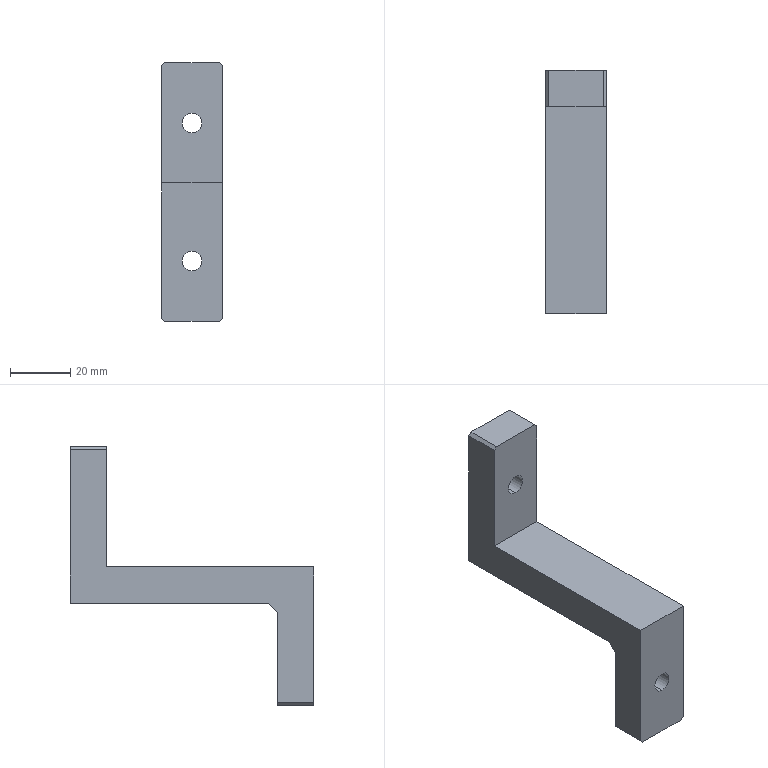Part | NX | features BREP 1 | 1 solid | 25 faces | box 20 x 81 x 86 mm | volume 35618 mm3 | plane 17 | cylinder 8 | commonest cylinder face diameters 6.6 x4 11 x4
STEP:
#1=CARTESIAN_POINT('',(9.,12.,0.));
#2=VERTEX_POINT('',#1);
#3=CARTESIAN_POINT('',(10.,12.,-1.));
#4=VERTEX_POINT('',#3);
#5=CARTESIAN_POINT('',(10.,12.,-1.));
#6=DIRECTION('',(0.7071,0.,-0.7071));
#7=VECTOR('',#6,1000.);
#8=LINE('',#5,#7);
#9=EDGE_CURVE('',#2,#4,#8,.T.);
#10=ORIENTED_EDGE('',*,*,#9,.F.);
#11=CARTESIAN_POINT('',(9.,0.,0.));
#12=VERTEX_POINT('',#11);
#13=CARTESIAN_POINT('',(9.,12.,0.));
#14=DIRECTION('',(0.,1.,0.));
#15=VECTOR('',#14,1000.);
#16=LINE('',#13,#15);
#17=EDGE_CURVE('',#12,#2,#16,.T.);
#18=ORIENTED_EDGE('',*,*,#17,.F.);
#19=CARTESIAN_POINT('',(10.,0.,-1.));
#20=VERTEX_POINT('',#19);
#21=CARTESIAN_POINT('',(10.,0.,-1.));
#22=DIRECTION('',(-0.7071,0.,0.7071));
#23=VECTOR('',#22,1000.);
#24=LINE('',#21,#23);
#25=EDGE_CURVE('',#20,#12,#24,.T.);
#26=ORIENTED_EDGE('',*,*,#25,.F.);
#27=CARTESIAN_POINT('',(10.,0.,-1.));
#28=DIRECTION('',(0.,-1.,0.));
#29=VECTOR('',#28,1000.);
#30=LINE('',#27,#29);
#31=EDGE_CURVE('',#4,#20,#30,.T.);
#32=ORIENTED_EDGE('',*,*,#31,.F.);
#33=EDGE_LOOP('',(#10,#18,#26,#32));
#34=FACE_BOUND('',#33,.T.);
#35=CARTESIAN_POINT('',(10.,0.,-1.));
#36=DIRECTION('',(0.7071,0.,0.7071));
#37=DIRECTION('',(0.,1.,0.));
#38=AXIS2_PLACEMENT_3D('',#35,#36,#37);
#39=PLANE('',#38);
#40=ADVANCED_FACE('',(#34),#39,.T.);
#41=CARTESIAN_POINT('',(-10.,12.,-1.));
#42=VERTEX_POINT('',#41);
#43=CARTESIAN_POINT('',(-9.,12.,0.));
#44=VERTEX_POINT('',#43);
#45=CARTESIAN_POINT('',(-9.,12.,0.));
#46=DIRECTION('',(0.7071,0.,0.7071));
#47=VECTOR('',#46,1000.);
#48=LINE('',#45,#47);
#49=EDGE_CURVE('',#42,#44,#48,.T.);
#50=ORIENTED_EDGE('',*,*,#49,.F.);
#51=CARTESIAN_POINT('',(-10.,0.,-1.));
#52=VERTEX_POINT('',#51);
#53=CARTESIAN_POINT('',(-10.,0.,-1.));
#54=DIRECTION('',(0.,1.,0.));
#55=VECTOR('',#54,1000.);
#56=LINE('',#53,#55);
#57=EDGE_CURVE('',#52,#42,#56,.T.);
#58=ORIENTED_EDGE('',*,*,#57,.F.);
#59=CARTESIAN_POINT('',(-9.,0.,0.));
#60=VERTEX_POINT('',#59);
#61=CARTESIAN_POINT('',(-9.,0.,0.));
#62=DIRECTION('',(-0.7071,0.,-0.7071));
#63=VECTOR('',#62,1000.);
#64=LINE('',#61,#63);
#65=EDGE_CURVE('',#60,#52,#64,.T.);
#66=ORIENTED_EDGE('',*,*,#65,.F.);
#67=CARTESIAN_POINT('',(-9.,12.,0.));
#68=DIRECTION('',(0.,-1.,0.));
#69=VECTOR('',#68,1000.);
#70=LINE('',#67,#69);
#71=EDGE_CURVE('',#44,#60,#70,.T.);
#72=ORIENTED_EDGE('',*,*,#71,.F.);
#73=EDGE_LOOP('',(#50,#58,#66,#72));
#74=FACE_BOUND('',#73,.T.);
#75=CARTESIAN_POINT('',(-9.,12.,0.));
#76=DIRECTION('',(0.7071,0.,-0.7071));
#77=DIRECTION('',(0.,-1.,0.));
#78=AXIS2_PLACEMENT_3D('',#75,#76,#77);
#79=PLANE('',#78);
#80=ADVANCED_FACE('',(#74),#79,.F.);
#81=CARTESIAN_POINT('',(9.,-69.,-86.));
#82=VERTEX_POINT('',#81);
#83=CARTESIAN_POINT('',(10.,-69.,-85.));
#84=VERTEX_POINT('',#83);
#85=CARTESIAN_POINT('',(10.,-69.,-85.));
#86=DIRECTION('',(0.7071,0.,0.7071));
#87=VECTOR('',#86,1000.);
#88=LINE('',#85,#87);
#89=EDGE_CURVE('',#82,#84,#88,.T.);
#90=ORIENTED_EDGE('',*,*,#89,.F.);
#91=CARTESIAN_POINT('',(9.,-57.,-86.));
#92=VERTEX_POINT('',#91);
#93=CARTESIAN_POINT('',(9.,-69.,-86.));
#94=DIRECTION('',(0.,-1.,0.));
#95=VECTOR('',#94,1000.);
#96=LINE('',#93,#95);
#97=EDGE_CURVE('',#92,#82,#96,.T.);
#98=ORIENTED_EDGE('',*,*,#97,.F.);
#99=CARTESIAN_POINT('',(10.,-57.,-85.));
#100=VERTEX_POINT('',#99);
#101=CARTESIAN_POINT('',(10.,-57.,-85.));
#102=DIRECTION('',(-0.7071,0.,-0.7071));
#103=VECTOR('',#102,1000.);
#104=LINE('',#101,#103);
#105=EDGE_CURVE('',#100,#92,#104,.T.);
#106=ORIENTED_EDGE('',*,*,#105,.F.);
#107=CARTESIAN_POINT('',(10.,-57.,-85.));
#108=DIRECTION('',(0.,1.,0.));
#109=VECTOR('',#108,1000.);
#110=LINE('',#107,#109);
#111=EDGE_CURVE('',#84,#100,#110,.T.);
#112=ORIENTED_EDGE('',*,*,#111,.F.);
#113=EDGE_LOOP('',(#90,#98,#106,#112));
#114=FACE_BOUND('',#113,.T.);
#115=CARTESIAN_POINT('',(10.,0.,-85.));
#116=DIRECTION('',(0.7071,0.,-0.7071));
#117=DIRECTION('',(0.,-1.,0.));
#118=AXIS2_PLACEMENT_3D('',#115,#116,#117);
#119=PLANE('',#118);
#120=ADVANCED_FACE('',(#114),#119,.T.);
#121=CARTESIAN_POINT('',(-10.,-69.,-85.));
#122=VERTEX_POINT('',#121);
#123=CARTESIAN_POINT('',(-9.,-69.,-86.));
#124=VERTEX_POINT('',#123);
#125=CARTESIAN_POINT('',(-9.,-69.,-86.));
#126=DIRECTION('',(0.7071,0.,-0.7071));
#127=VECTOR('',#126,1000.);
#128=LINE('',#125,#127);
#129=EDGE_CURVE('',#122,#124,#128,.T.);
#130=ORIENTED_EDGE('',*,*,#129,.F.);
#131=CARTESIAN_POINT('',(-10.,-57.,-85.));
#132=VERTEX_POINT('',#131);
#133=CARTESIAN_POINT('',(-10.,0.,-85.));
#134=DIRECTION('',(0.,-1.,0.));
#135=VECTOR('',#134,1000.);
#136=LINE('',#133,#135);
#137=EDGE_CURVE('',#132,#122,#136,.T.);
#138=ORIENTED_EDGE('',*,*,#137,.F.);
#139=CARTESIAN_POINT('',(-9.,-57.,-86.));
#140=VERTEX_POINT('',#139);
#141=CARTESIAN_POINT('',(-9.,-57.,-86.));
#142=DIRECTION('',(-0.7071,0.,0.7071));
#143=VECTOR('',#142,1000.);
#144=LINE('',#141,#143);
#145=EDGE_CURVE('',#140,#132,#144,.T.);
#146=ORIENTED_EDGE('',*,*,#145,.F.);
#147=CARTESIAN_POINT('',(-9.,-69.,-86.));
#148=DIRECTION('',(0.,1.,0.));
#149=VECTOR('',#148,1000.);
#150=LINE('',#147,#149);
#151=EDGE_CURVE('',#124,#140,#150,.T.);
#152=ORIENTED_EDGE('',*,*,#151,.F.);
#153=EDGE_LOOP('',(#130,#138,#146,#152));
#154=FACE_BOUND('',#153,.T.);
#155=CARTESIAN_POINT('',(-9.,-69.,-86.));
#156=DIRECTION('',(0.7071,0.,0.7071));
#157=DIRECTION('',(0.,1.,0.));
#158=AXIS2_PLACEMENT_3D('',#155,#156,#157);
#159=PLANE('',#158);
#160=ADVANCED_FACE('',(#154),#159,.F.);
#161=CARTESIAN_POINT('',(0.,-57.,-71.5));
#162=VERTEX_POINT('',#161);
#163=CARTESIAN_POINT('',(0.,-63.8,-71.5));
#164=VERTEX_POINT('',#163);
#165=CARTESIAN_POINT('',(0.,-57.,-71.5));
#166=DIRECTION('',(0.,1.,0.));
#167=VECTOR('',#166,1000.);
#168=LINE('',#165,#167);
#169=EDGE_CURVE('',#162,#164,#168,.F.);
#170=ORIENTED_EDGE('',*,*,#169,.T.);
#171=CARTESIAN_POINT('',(0.,-63.8,-60.5));
#172=VERTEX_POINT('',#171);
#173=CARTESIAN_POINT('',(0.,-63.8,-66.));
#174=DIRECTION('',(0.,1.,0.));
#175=DIRECTION('',(0.,0.,1.));
#176=AXIS2_PLACEMENT_3D('',#173,#174,#175);
#177=CIRCLE('',#176,5.5);
#178=EDGE_CURVE('',#172,#164,#177,.T.);
#179=ORIENTED_EDGE('',*,*,#178,.F.);
#180=CARTESIAN_POINT('',(0.,-57.,-60.5));
#181=VERTEX_POINT('',#180);
#182=CARTESIAN_POINT('',(0.,-57.,-60.5));
#183=DIRECTION('',(0.,1.,0.));
#184=VECTOR('',#183,1000.);
#185=LINE('',#182,#184);
#186=EDGE_CURVE('',#181,#172,#185,.F.);
#187=ORIENTED_EDGE('',*,*,#186,.F.);
#188=CARTESIAN_POINT('',(0.,-57.,-66.));
#189=DIRECTION('',(0.,1.,0.));
#190=DIRECTION('',(0.,0.,1.));
#191=AXIS2_PLACEMENT_3D('',#188,#189,#190);
#192=CIRCLE('',#191,5.5);
#193=EDGE_CURVE('',#181,#162,#192,.T.);
#194=ORIENTED_EDGE('',*,*,#193,.T.);
#195=EDGE_LOOP('',(#170,#179,#187,#194));
#196=FACE_BOUND('',#195,.T.);
#197=CARTESIAN_POINT('',(0.,-57.,-66.));
#198=DIRECTION('',(0.,1.,0.));
#199=DIRECTION('',(0.,0.,1.));
#200=AXIS2_PLACEMENT_3D('',#197,#198,#199);
#201=CYLINDRICAL_SURFACE('',#200,5.5);
#202=ADVANCED_FACE('',(#196),#201,.F.);
#203=ORIENTED_EDGE('',*,*,#178,.T.);
#204=CARTESIAN_POINT('',(0.,-63.8,-66.));
#205=DIRECTION('',(0.,1.,0.));
#206=DIRECTION('',(0.,0.,1.));
#207=AXIS2_PLACEMENT_3D('',#204,#205,#206);
#208=CIRCLE('',#207,5.5);
#209=EDGE_CURVE('',#164,#172,#208,.T.);
#210=ORIENTED_EDGE('',*,*,#209,.T.);
#211=EDGE_LOOP('',(#203,#210));
#212=FACE_BOUND('',#211,.T.);
#213=CARTESIAN_POINT('',(0.,-63.8,-62.7));
#214=VERTEX_POINT('',#213);
#215=CARTESIAN_POINT('',(0.,-63.8,-69.3));
#216=VERTEX_POINT('',#215);
#217=CARTESIAN_POINT('',(0.,-63.8,-66.));
#218=DIRECTION('',(0.,1.,0.));
#219=DIRECTION('',(0.,0.,1.));
#220=AXIS2_PLACEMENT_3D('',#217,#218,#219);
#221=CIRCLE('',#220,3.3);
#222=EDGE_CURVE('',#214,#216,#221,.T.);
#223=ORIENTED_EDGE('',*,*,#222,.F.);
#224=CARTESIAN_POINT('',(0.,-63.8,-66.));
#225=DIRECTION('',(0.,1.,0.));
#226=DIRECTION('',(0.,0.,1.));
#227=AXIS2_PLACEMENT_3D('',#224,#225,#226);
#228=CIRCLE('',#227,3.3);
#229=EDGE_CURVE('',#216,#214,#228,.T.);
#230=ORIENTED_EDGE('',*,*,#229,.F.);
#231=EDGE_LOOP('',(#223,#230));
#232=FACE_BOUND('',#231,.T.);
#233=CARTESIAN_POINT('',(3.3,-63.8,-66.));
#234=DIRECTION('',(0.,-1.,0.));
#235=DIRECTION('',(0.,0.,-1.));
#236=AXIS2_PLACEMENT_3D('',#233,#234,#235);
#237=PLANE('',#236);
#238=ADVANCED_FACE('',(#212,#232),#237,.F.);
#239=CARTESIAN_POINT('',(0.,-69.,-69.3));
#240=VERTEX_POINT('',#239);
#241=CARTESIAN_POINT('',(0.,-57.,-69.3));
#242=DIRECTION('',(0.,1.,0.));
#243=VECTOR('',#242,1000.);
#244=LINE('',#241,#243);
#245=EDGE_CURVE('',#216,#240,#244,.F.);
#246=ORIENTED_EDGE('',*,*,#245,.T.);
#247=CARTESIAN_POINT('',(0.,-69.,-62.7));
#248=VERTEX_POINT('',#247);
#249=CARTESIAN_POINT('',(0.,-69.,-66.));
#250=DIRECTION('',(0.,1.,0.));
#251=DIRECTION('',(0.,0.,1.));
#252=AXIS2_PLACEMENT_3D('',#249,#250,#251);
#253=CIRCLE('',#252,3.3);
#254=EDGE_CURVE('',#248,#240,#253,.T.);
#255=ORIENTED_EDGE('',*,*,#254,.F.);
#256=CARTESIAN_POINT('',(0.,-57.,-62.7));
#257=DIRECTION('',(0.,1.,0.));
#258=VECTOR('',#257,1000.);
#259=LINE('',#256,#258);
#260=EDGE_CURVE('',#214,#248,#259,.F.);
#261=ORIENTED_EDGE('',*,*,#260,.F.);
#262=ORIENTED_EDGE('',*,*,#222,.T.);
#263=EDGE_LOOP('',(#246,#255,#261,#262));
#264=FACE_BOUND('',#263,.T.);
#265=CARTESIAN_POINT('',(0.,-57.,-66.));
#266=DIRECTION('',(0.,1.,0.));
#267=DIRECTION('',(0.,0.,1.));
#268=AXIS2_PLACEMENT_3D('',#265,#266,#267);
#269=CYLINDRICAL_SURFACE('',#268,3.3);
#270=ADVANCED_FACE('',(#264),#269,.F.);
#271=CARTESIAN_POINT('',(10.,-57.,-55.));
#272=VERTEX_POINT('',#271);
#273=CARTESIAN_POINT('',(10.,-54.,-52.));
#274=VERTEX_POINT('',#273);
#275=CARTESIAN_POINT('',(10.,-54.,-52.));
#276=DIRECTION('',(0.,0.7071,0.7071));
#277=VECTOR('',#276,1000.);
#278=LINE('',#275,#277);
#279=EDGE_CURVE('',#272,#274,#278,.T.);
#280=ORIENTED_EDGE('',*,*,#279,.F.);
#281=CARTESIAN_POINT('',(-10.,-57.,-55.));
#282=VERTEX_POINT('',#281);
#283=CARTESIAN_POINT('',(10.,-57.,-55.));
#284=DIRECTION('',(1.,0.,0.));
#285=VECTOR('',#284,1000.);
#286=LINE('',#283,#285);
#287=EDGE_CURVE('',#282,#272,#286,.T.);
#288=ORIENTED_EDGE('',*,*,#287,.F.);
#289=CARTESIAN_POINT('',(-10.,-54.,-52.));
#290=VERTEX_POINT('',#289);
#291=CARTESIAN_POINT('',(-10.,-1.,1.));
#292=DIRECTION('',(0.,-0.7071,-0.7071));
#293=VECTOR('',#292,1000.);
#294=LINE('',#291,#293);
#295=EDGE_CURVE('',#290,#282,#294,.T.);
#296=ORIENTED_EDGE('',*,*,#295,.F.);
#297=CARTESIAN_POINT('',(-10.,-54.,-52.));
#298=DIRECTION('',(-1.,0.,0.));
#299=VECTOR('',#298,1000.);
#300=LINE('',#297,#299);
#301=EDGE_CURVE('',#274,#290,#300,.T.);
#302=ORIENTED_EDGE('',*,*,#301,.F.);
#303=EDGE_LOOP('',(#280,#288,#296,#302));
#304=FACE_BOUND('',#303,.T.);
#305=CARTESIAN_POINT('',(10.,-54.,-52.));
#306=DIRECTION('',(0.,0.7071,-0.7071));
#307=DIRECTION('',(1.,0.,0.));
#308=AXIS2_PLACEMENT_3D('',#305,#306,#307);
#309=PLANE('',#308);
#310=ADVANCED_FACE('',(#304),#309,.T.);
#311=CARTESIAN_POINT('',(0.,12.,-25.5));
#312=VERTEX_POINT('',#311);
#313=CARTESIAN_POINT('',(0.,5.2,-25.5));
#314=VERTEX_POINT('',#313);
#315=CARTESIAN_POINT('',(0.,12.,-25.5));
#316=DIRECTION('',(0.,1.,0.));
#317=VECTOR('',#316,1000.);
#318=LINE('',#315,#317);
#319=EDGE_CURVE('',#312,#314,#318,.F.);
#320=ORIENTED_EDGE('',*,*,#319,.T.);
#321=CARTESIAN_POINT('',(0.,5.2,-14.5));
#322=VERTEX_POINT('',#321);
#323=CARTESIAN_POINT('',(0.,5.2,-20.));
#324=DIRECTION('',(0.,1.,0.));
#325=DIRECTION('',(0.,0.,1.));
#326=AXIS2_PLACEMENT_3D('',#323,#324,#325);
#327=CIRCLE('',#326,5.5);
#328=EDGE_CURVE('',#322,#314,#327,.T.);
#329=ORIENTED_EDGE('',*,*,#328,.F.);
#330=CARTESIAN_POINT('',(0.,12.,-14.5));
#331=VERTEX_POINT('',#330);
#332=CARTESIAN_POINT('',(0.,12.,-14.5));
#333=DIRECTION('',(0.,1.,0.));
#334=VECTOR('',#333,1000.);
#335=LINE('',#332,#334);
#336=EDGE_CURVE('',#331,#322,#335,.F.);
#337=ORIENTED_EDGE('',*,*,#336,.F.);
#338=CARTESIAN_POINT('',(0.,12.,-20.));
#339=DIRECTION('',(0.,1.,0.));
#340=DIRECTION('',(0.,0.,1.));
#341=AXIS2_PLACEMENT_3D('',#338,#339,#340);
#342=CIRCLE('',#341,5.5);
#343=EDGE_CURVE('',#331,#312,#342,.T.);
#344=ORIENTED_EDGE('',*,*,#343,.T.);
#345=EDGE_LOOP('',(#320,#329,#337,#344));
#346=FACE_BOUND('',#345,.T.);
#347=CARTESIAN_POINT('',(0.,12.,-20.));
#348=DIRECTION('',(0.,1.,0.));
#349=DIRECTION('',(0.,0.,1.));
#350=AXIS2_PLACEMENT_3D('',#347,#348,#349);
#351=CYLINDRICAL_SURFACE('',#350,5.5);
#352=ADVANCED_FACE('',(#346),#351,.F.);
#353=ORIENTED_EDGE('',*,*,#328,.T.);
#354=CARTESIAN_POINT('',(0.,5.2,-20.));
#355=DIRECTION('',(0.,1.,0.));
#356=DIRECTION('',(0.,0.,1.));
#357=AXIS2_PLACEMENT_3D('',#354,#355,#356);
#358=CIRCLE('',#357,5.5);
#359=EDGE_CURVE('',#314,#322,#358,.T.);
#360=ORIENTED_EDGE('',*,*,#359,.T.);
#361=EDGE_LOOP('',(#353,#360));
#362=FACE_BOUND('',#361,.T.);
#363=CARTESIAN_POINT('',(0.,5.2,-16.7));
#364=VERTEX_POINT('',#363);
#365=CARTESIAN_POINT('',(0.,5.2,-23.3));
#366=VERTEX_POINT('',#365);
#367=CARTESIAN_POINT('',(0.,5.2,-20.));
#368=DIRECTION('',(0.,1.,0.));
#369=DIRECTION('',(0.,0.,1.));
#370=AXIS2_PLACEMENT_3D('',#367,#368,#369);
#371=CIRCLE('',#370,3.3);
#372=EDGE_CURVE('',#364,#366,#371,.T.);
#373=ORIENTED_EDGE('',*,*,#372,.F.);
#374=CARTESIAN_POINT('',(0.,5.2,-20.));
#375=DIRECTION('',(0.,1.,0.));
#376=DIRECTION('',(0.,0.,1.));
#377=AXIS2_PLACEMENT_3D('',#374,#375,#376);
#378=CIRCLE('',#377,3.3);
#379=EDGE_CURVE('',#366,#364,#378,.T.);
#380=ORIENTED_EDGE('',*,*,#379,.F.);
#381=EDGE_LOOP('',(#373,#380));
#382=FACE_BOUND('',#381,.T.);
#383=CARTESIAN_POINT('',(3.3,5.2,-20.));
#384=DIRECTION('',(0.,-1.,0.));
#385=DIRECTION('',(0.,0.,-1.));
#386=AXIS2_PLACEMENT_3D('',#383,#384,#385);
#387=PLANE('',#386);
#388=ADVANCED_FACE('',(#362,#382),#387,.F.);
#389=CARTESIAN_POINT('',(0.,0.,-23.3));
#390=VERTEX_POINT('',#389);
#391=CARTESIAN_POINT('',(0.,12.,-23.3));
#392=DIRECTION('',(0.,1.,0.));
#393=VECTOR('',#392,1000.);
#394=LINE('',#391,#393);
#395=EDGE_CURVE('',#366,#390,#394,.F.);
#396=ORIENTED_EDGE('',*,*,#395,.T.);
#397=CARTESIAN_POINT('',(0.,0.,-16.7));
#398=VERTEX_POINT('',#397);
#399=CARTESIAN_POINT('',(0.,0.,-20.));
#400=DIRECTION('',(0.,1.,0.));
#401=DIRECTION('',(0.,0.,1.));
#402=AXIS2_PLACEMENT_3D('',#399,#400,#401);
#403=CIRCLE('',#402,3.3);
#404=EDGE_CURVE('',#398,#390,#403,.T.);
#405=ORIENTED_EDGE('',*,*,#404,.F.);
#406=CARTESIAN_POINT('',(0.,12.,-16.7));
#407=DIRECTION('',(0.,1.,0.));
#408=VECTOR('',#407,1000.);
#409=LINE('',#406,#408);
#410=EDGE_CURVE('',#364,#398,#409,.F.);
#411=ORIENTED_EDGE('',*,*,#410,.F.);
#412=ORIENTED_EDGE('',*,*,#372,.T.);
#413=EDGE_LOOP('',(#396,#405,#411,#412));
#414=FACE_BOUND('',#413,.T.);
#415=CARTESIAN_POINT('',(0.,12.,-20.));
#416=DIRECTION('',(0.,1.,0.));
#417=DIRECTION('',(0.,0.,1.));
#418=AXIS2_PLACEMENT_3D('',#415,#416,#417);
#419=CYLINDRICAL_SURFACE('',#418,3.3);
#420=ADVANCED_FACE('',(#414),#419,.F.);
#421=CARTESIAN_POINT('',(-10.,-57.,-86.));
#422=DIRECTION('',(0.,0.,1.));
#423=VECTOR('',#422,1000.);
#424=LINE('',#421,#423);
#425=EDGE_CURVE('',#132,#282,#424,.T.);
#426=ORIENTED_EDGE('',*,*,#425,.F.);
#427=ORIENTED_EDGE('',*,*,#137,.T.);
#428=CARTESIAN_POINT('',(-10.,-69.,-40.));
#429=VERTEX_POINT('',#428);
#430=CARTESIAN_POINT('',(-10.,-69.,-40.));
#431=DIRECTION('',(0.,0.,-1.));
#432=VECTOR('',#431,1000.);
#433=LINE('',#430,#432);
#434=EDGE_CURVE('',#429,#122,#433,.T.);
#435=ORIENTED_EDGE('',*,*,#434,.F.);
#436=CARTESIAN_POINT('',(-10.,0.,-40.));
#437=VERTEX_POINT('',#436);
#438=CARTESIAN_POINT('',(-10.,0.,-40.));
#439=DIRECTION('',(0.,-1.,0.));
#440=VECTOR('',#439,1000.);
#441=LINE('',#438,#440);
#442=EDGE_CURVE('',#437,#429,#441,.T.);
#443=ORIENTED_EDGE('',*,*,#442,.F.);
#444=CARTESIAN_POINT('',(-10.,0.,0.));
#445=DIRECTION('',(0.,0.,-1.));
#446=VECTOR('',#445,1000.);
#447=LINE('',#444,#446);
#448=EDGE_CURVE('',#52,#437,#447,.T.);
#449=ORIENTED_EDGE('',*,*,#448,.F.);
#450=ORIENTED_EDGE('',*,*,#57,.T.);
#451=CARTESIAN_POINT('',(-10.,12.,-52.));
#452=VERTEX_POINT('',#451);
#453=CARTESIAN_POINT('',(-10.,12.,-52.));
#454=DIRECTION('',(0.,0.,1.));
#455=VECTOR('',#454,1000.);
#456=LINE('',#453,#455);
#457=EDGE_CURVE('',#452,#42,#456,.T.);
#458=ORIENTED_EDGE('',*,*,#457,.F.);
#459=CARTESIAN_POINT('',(-10.,-57.,-52.));
#460=DIRECTION('',(0.,1.,0.));
#461=VECTOR('',#460,1000.);
#462=LINE('',#459,#461);
#463=EDGE_CURVE('',#290,#452,#462,.T.);
#464=ORIENTED_EDGE('',*,*,#463,.F.);
#465=ORIENTED_EDGE('',*,*,#295,.T.);
#466=EDGE_LOOP('',(#426,#427,#435,#443,#449,#450,#458,#464,#465));
#467=FACE_BOUND('',#466,.T.);
#468=CARTESIAN_POINT('',(-10.,0.,0.));
#469=DIRECTION('',(1.,0.,0.));
#470=DIRECTION('',(0.,0.,-1.));
#471=AXIS2_PLACEMENT_3D('',#468,#469,#470);
#472=PLANE('',#471);
#473=ADVANCED_FACE('',(#467),#472,.F.);
#474=CARTESIAN_POINT('',(10.,-69.,-40.));
#475=VERTEX_POINT('',#474);
#476=CARTESIAN_POINT('',(10.,-69.,-40.));
#477=DIRECTION('',(0.,0.,-1.));
#478=VECTOR('',#477,1000.);
#479=LINE('',#476,#478);
#480=EDGE_CURVE('',#475,#84,#479,.T.);
#481=ORIENTED_EDGE('',*,*,#480,.T.);
#482=ORIENTED_EDGE('',*,*,#111,.T.);
#483=CARTESIAN_POINT('',(10.,-57.,-86.));
#484=DIRECTION('',(0.,0.,1.));
#485=VECTOR('',#484,1000.);
#486=LINE('',#483,#485);
#487=EDGE_CURVE('',#100,#272,#486,.T.);
#488=ORIENTED_EDGE('',*,*,#487,.T.);
#489=ORIENTED_EDGE('',*,*,#279,.T.);
#490=CARTESIAN_POINT('',(10.,12.,-52.));
#491=VERTEX_POINT('',#490);
#492=CARTESIAN_POINT('',(10.,-57.,-52.));
#493=DIRECTION('',(0.,1.,0.));
#494=VECTOR('',#493,1000.);
#495=LINE('',#492,#494);
#496=EDGE_CURVE('',#274,#491,#495,.T.);
#497=ORIENTED_EDGE('',*,*,#496,.T.);
#498=CARTESIAN_POINT('',(10.,12.,-52.));
#499=DIRECTION('',(0.,0.,1.));
#500=VECTOR('',#499,1000.);
#501=LINE('',#498,#500);
#502=EDGE_CURVE('',#491,#4,#501,.T.);
#503=ORIENTED_EDGE('',*,*,#502,.T.);
#504=ORIENTED_EDGE('',*,*,#31,.T.);
#505=CARTESIAN_POINT('',(10.,0.,-40.));
#506=VERTEX_POINT('',#505);
#507=CARTESIAN_POINT('',(10.,0.,0.));
#508=DIRECTION('',(0.,0.,-1.));
#509=VECTOR('',#508,1000.);
#510=LINE('',#507,#509);
#511=EDGE_CURVE('',#20,#506,#510,.T.);
#512=ORIENTED_EDGE('',*,*,#511,.T.);
#513=CARTESIAN_POINT('',(10.,0.,-40.));
#514=DIRECTION('',(0.,-1.,0.));
#515=VECTOR('',#514,1000.);
#516=LINE('',#513,#515);
#517=EDGE_CURVE('',#506,#475,#516,.T.);
#518=ORIENTED_EDGE('',*,*,#517,.T.);
#519=EDGE_LOOP('',(#481,#482,#488,#489,#497,#503,#504,#512,#518));
#520=FACE_BOUND('',#519,.T.);
#521=CARTESIAN_POINT('',(10.,0.,0.));
#522=DIRECTION('',(1.,0.,0.));
#523=DIRECTION('',(0.,0.,-1.));
#524=AXIS2_PLACEMENT_3D('',#521,#522,#523);
#525=PLANE('',#524);
#526=ADVANCED_FACE('',(#520),#525,.T.);
#527=ORIENTED_EDGE('',*,*,#457,.T.);
#528=ORIENTED_EDGE('',*,*,#49,.T.);
#529=CARTESIAN_POINT('',(10.,12.,0.));
#530=DIRECTION('',(-1.,0.,0.));
#531=VECTOR('',#530,1000.);
#532=LINE('',#529,#531);
#533=EDGE_CURVE('',#2,#44,#532,.T.);
#534=ORIENTED_EDGE('',*,*,#533,.F.);
#535=ORIENTED_EDGE('',*,*,#9,.T.);
#536=ORIENTED_EDGE('',*,*,#502,.F.);
#537=CARTESIAN_POINT('',(10.,12.,-52.));
#538=DIRECTION('',(-1.,0.,0.));
#539=VECTOR('',#538,1000.);
#540=LINE('',#537,#539);
#541=EDGE_CURVE('',#491,#452,#540,.T.);
#542=ORIENTED_EDGE('',*,*,#541,.T.);
#543=EDGE_LOOP('',(#527,#528,#534,#535,#536,#542));
#544=FACE_BOUND('',#543,.T.);
#545=ORIENTED_EDGE('',*,*,#343,.F.);
#546=CARTESIAN_POINT('',(0.,12.,-20.));
#547=DIRECTION('',(0.,1.,0.));
#548=DIRECTION('',(0.,0.,1.));
#549=AXIS2_PLACEMENT_3D('',#546,#547,#548);
#550=CIRCLE('',#549,5.5);
#551=EDGE_CURVE('',#312,#331,#550,.T.);
#552=ORIENTED_EDGE('',*,*,#551,.F.);
#553=EDGE_LOOP('',(#545,#552));
#554=FACE_BOUND('',#553,.T.);
#555=CARTESIAN_POINT('',(10.,12.,-52.));
#556=DIRECTION('',(0.,-1.,0.));
#557=DIRECTION('',(0.,0.,-1.));
#558=AXIS2_PLACEMENT_3D('',#555,#556,#557);
#559=PLANE('',#558);
#560=ADVANCED_FACE('',(#544,#554),#559,.F.);
#561=ORIENTED_EDGE('',*,*,#496,.F.);
#562=ORIENTED_EDGE('',*,*,#301,.T.);
#563=ORIENTED_EDGE('',*,*,#463,.T.);
#564=ORIENTED_EDGE('',*,*,#541,.F.);
#565=EDGE_LOOP('',(#561,#562,#563,#564));
#566=FACE_BOUND('',#565,.T.);
#567=CARTESIAN_POINT('',(10.,-57.,-52.));
#568=DIRECTION('',(0.,0.,1.));
#569=DIRECTION('',(1.,0.,0.));
#570=AXIS2_PLACEMENT_3D('',#567,#568,#569);
#571=PLANE('',#570);
#572=ADVANCED_FACE('',(#566),#571,.F.);
#573=CARTESIAN_POINT('',(10.,-57.,-86.));
#574=DIRECTION('',(-1.,0.,0.));
#575=VECTOR('',#574,1000.);
#576=LINE('',#573,#575);
#577=EDGE_CURVE('',#92,#140,#576,.T.);
#578=ORIENTED_EDGE('',*,*,#577,.T.);
#579=ORIENTED_EDGE('',*,*,#145,.T.);
#580=ORIENTED_EDGE('',*,*,#425,.T.);
#581=ORIENTED_EDGE('',*,*,#287,.T.);
#582=ORIENTED_EDGE('',*,*,#487,.F.);
#583=ORIENTED_EDGE('',*,*,#105,.T.);
#584=EDGE_LOOP('',(#578,#579,#580,#581,#582,#583));
#585=FACE_BOUND('',#584,.T.);
#586=ORIENTED_EDGE('',*,*,#193,.F.);
#587=CARTESIAN_POINT('',(0.,-57.,-66.));
#588=DIRECTION('',(0.,1.,0.));
#589=DIRECTION('',(0.,0.,1.));
#590=AXIS2_PLACEMENT_3D('',#587,#588,#589);
#591=CIRCLE('',#590,5.5);
#592=EDGE_CURVE('',#162,#181,#591,.T.);
#593=ORIENTED_EDGE('',*,*,#592,.F.);
#594=EDGE_LOOP('',(#586,#593));
#595=FACE_BOUND('',#594,.T.);
#596=CARTESIAN_POINT('',(10.,-57.,-86.));
#597=DIRECTION('',(0.,-1.,0.));
#598=DIRECTION('',(0.,0.,-1.));
#599=AXIS2_PLACEMENT_3D('',#596,#597,#598);
#600=PLANE('',#599);
#601=ADVANCED_FACE('',(#585,#595),#600,.F.);
#602=CARTESIAN_POINT('',(10.,-69.,-86.));
#603=DIRECTION('',(-1.,0.,0.));
#604=VECTOR('',#603,1000.);
#605=LINE('',#602,#604);
#606=EDGE_CURVE('',#82,#124,#605,.T.);
#607=ORIENTED_EDGE('',*,*,#606,.T.);
#608=ORIENTED_EDGE('',*,*,#151,.T.);
#609=ORIENTED_EDGE('',*,*,#577,.F.);
#610=ORIENTED_EDGE('',*,*,#97,.T.);
#611=EDGE_LOOP('',(#607,#608,#609,#610));
#612=FACE_BOUND('',#611,.T.);
#613=CARTESIAN_POINT('',(10.,-69.,-86.));
#614=DIRECTION('',(0.,0.,1.));
#615=DIRECTION('',(1.,0.,0.));
#616=AXIS2_PLACEMENT_3D('',#613,#614,#615);
#617=PLANE('',#616);
#618=ADVANCED_FACE('',(#612),#617,.F.);
#619=ORIENTED_EDGE('',*,*,#434,.T.);
#620=ORIENTED_EDGE('',*,*,#129,.T.);
#621=ORIENTED_EDGE('',*,*,#606,.F.);
#622=ORIENTED_EDGE('',*,*,#89,.T.);
#623=ORIENTED_EDGE('',*,*,#480,.F.);
#624=CARTESIAN_POINT('',(10.,-69.,-40.));
#625=DIRECTION('',(-1.,0.,0.));
#626=VECTOR('',#625,1000.);
#627=LINE('',#624,#626);
#628=EDGE_CURVE('',#475,#429,#627,.T.);
#629=ORIENTED_EDGE('',*,*,#628,.T.);
#630=EDGE_LOOP('',(#619,#620,#621,#622,#623,#629));
#631=FACE_BOUND('',#630,.T.);
#632=ORIENTED_EDGE('',*,*,#254,.T.);
#633=CARTESIAN_POINT('',(0.,-69.,-66.));
#634=DIRECTION('',(0.,1.,0.));
#635=DIRECTION('',(0.,0.,1.));
#636=AXIS2_PLACEMENT_3D('',#633,#634,#635);
#637=CIRCLE('',#636,3.3);
#638=EDGE_CURVE('',#240,#248,#637,.T.);
#639=ORIENTED_EDGE('',*,*,#638,.T.);
#640=EDGE_LOOP('',(#632,#639));
#641=FACE_BOUND('',#640,.T.);
#642=CARTESIAN_POINT('',(10.,-69.,-40.));
#643=DIRECTION('',(0.,1.,0.));
#644=DIRECTION('',(0.,0.,1.));
#645=AXIS2_PLACEMENT_3D('',#642,#643,#644);
#646=PLANE('',#645);
#647=ADVANCED_FACE('',(#631,#641),#646,.F.);
#648=ORIENTED_EDGE('',*,*,#442,.T.);
#649=ORIENTED_EDGE('',*,*,#628,.F.);
#650=ORIENTED_EDGE('',*,*,#517,.F.);
#651=CARTESIAN_POINT('',(10.,0.,-40.));
#652=DIRECTION('',(-1.,0.,0.));
#653=VECTOR('',#652,1000.);
#654=LINE('',#651,#653);
#655=EDGE_CURVE('',#506,#437,#654,.T.);
#656=ORIENTED_EDGE('',*,*,#655,.T.);
#657=EDGE_LOOP('',(#648,#649,#650,#656));
#658=FACE_BOUND('',#657,.T.);
#659=CARTESIAN_POINT('',(10.,0.,-40.));
#660=DIRECTION('',(0.,0.,-1.));
#661=DIRECTION('',(0.,1.,0.));
#662=AXIS2_PLACEMENT_3D('',#659,#660,#661);
#663=PLANE('',#662);
#664=ADVANCED_FACE('',(#658),#663,.F.);
#665=CARTESIAN_POINT('',(10.,0.,0.));
#666=DIRECTION('',(-1.,0.,0.));
#667=VECTOR('',#666,1000.);
#668=LINE('',#665,#667);
#669=EDGE_CURVE('',#12,#60,#668,.T.);
#670=ORIENTED_EDGE('',*,*,#669,.T.);
#671=ORIENTED_EDGE('',*,*,#65,.T.);
#672=ORIENTED_EDGE('',*,*,#448,.T.);
#673=ORIENTED_EDGE('',*,*,#655,.F.);
#674=ORIENTED_EDGE('',*,*,#511,.F.);
#675=ORIENTED_EDGE('',*,*,#25,.T.);
#676=EDGE_LOOP('',(#670,#671,#672,#673,#674,#675));
#677=FACE_BOUND('',#676,.T.);
#678=ORIENTED_EDGE('',*,*,#404,.T.);
#679=CARTESIAN_POINT('',(0.,0.,-20.));
#680=DIRECTION('',(0.,1.,0.));
#681=DIRECTION('',(0.,0.,1.));
#682=AXIS2_PLACEMENT_3D('',#679,#680,#681);
#683=CIRCLE('',#682,3.3);
#684=EDGE_CURVE('',#390,#398,#683,.T.);
#685=ORIENTED_EDGE('',*,*,#684,.T.);
#686=EDGE_LOOP('',(#678,#685));
#687=FACE_BOUND('',#686,.T.);
#688=CARTESIAN_POINT('',(10.,0.,0.));
#689=DIRECTION('',(0.,1.,0.));
#690=DIRECTION('',(0.,0.,1.));
#691=AXIS2_PLACEMENT_3D('',#688,#689,#690);
#692=PLANE('',#691);
#693=ADVANCED_FACE('',(#677,#687),#692,.F.);
#694=ORIENTED_EDGE('',*,*,#533,.T.);
#695=ORIENTED_EDGE('',*,*,#71,.T.);
#696=ORIENTED_EDGE('',*,*,#669,.F.);
#697=ORIENTED_EDGE('',*,*,#17,.T.);
#698=EDGE_LOOP('',(#694,#695,#696,#697));
#699=FACE_BOUND('',#698,.T.);
#700=CARTESIAN_POINT('',(10.,12.,0.));
#701=DIRECTION('',(0.,0.,-1.));
#702=DIRECTION('',(-1.,0.,0.));
#703=AXIS2_PLACEMENT_3D('',#700,#701,#702);
#704=PLANE('',#703);
#705=ADVANCED_FACE('',(#699),#704,.F.);
#706=ORIENTED_EDGE('',*,*,#684,.F.);
#707=ORIENTED_EDGE('',*,*,#395,.F.);
#708=ORIENTED_EDGE('',*,*,#379,.T.);
#709=ORIENTED_EDGE('',*,*,#410,.T.);
#710=EDGE_LOOP('',(#706,#707,#708,#709));
#711=FACE_BOUND('',#710,.T.);
#712=CARTESIAN_POINT('',(0.,12.,-20.));
#713=DIRECTION('',(0.,1.,0.));
#714=DIRECTION('',(0.,0.,1.));
#715=AXIS2_PLACEMENT_3D('',#712,#713,#714);
#716=CYLINDRICAL_SURFACE('',#715,3.3);
#717=ADVANCED_FACE('',(#711),#716,.F.);
#718=ORIENTED_EDGE('',*,*,#359,.F.);
#719=ORIENTED_EDGE('',*,*,#319,.F.);
#720=ORIENTED_EDGE('',*,*,#551,.T.);
#721=ORIENTED_EDGE('',*,*,#336,.T.);
#722=EDGE_LOOP('',(#718,#719,#720,#721));
#723=FACE_BOUND('',#722,.T.);
#724=CARTESIAN_POINT('',(0.,12.,-20.));
#725=DIRECTION('',(0.,1.,0.));
#726=DIRECTION('',(0.,0.,1.));
#727=AXIS2_PLACEMENT_3D('',#724,#725,#726);
#728=CYLINDRICAL_SURFACE('',#727,5.5);
#729=ADVANCED_FACE('',(#723),#728,.F.);
#730=ORIENTED_EDGE('',*,*,#638,.F.);
#731=ORIENTED_EDGE('',*,*,#245,.F.);
#732=ORIENTED_EDGE('',*,*,#229,.T.);
#733=ORIENTED_EDGE('',*,*,#260,.T.);
#734=EDGE_LOOP('',(#730,#731,#732,#733));
#735=FACE_BOUND('',#734,.T.);
#736=CARTESIAN_POINT('',(0.,-57.,-66.));
#737=DIRECTION('',(0.,1.,0.));
#738=DIRECTION('',(0.,0.,1.));
#739=AXIS2_PLACEMENT_3D('',#736,#737,#738);
#740=CYLINDRICAL_SURFACE('',#739,3.3);
#741=ADVANCED_FACE('',(#735),#740,.F.);
#742=ORIENTED_EDGE('',*,*,#209,.F.);
#743=ORIENTED_EDGE('',*,*,#169,.F.);
#744=ORIENTED_EDGE('',*,*,#592,.T.);
#745=ORIENTED_EDGE('',*,*,#186,.T.);
#746=EDGE_LOOP('',(#742,#743,#744,#745));
#747=FACE_BOUND('',#746,.T.);
#748=CARTESIAN_POINT('',(0.,-57.,-66.));
#749=DIRECTION('',(0.,1.,0.));
#750=DIRECTION('',(0.,0.,1.));
#751=AXIS2_PLACEMENT_3D('',#748,#749,#750);
#752=CYLINDRICAL_SURFACE('',#751,5.5);
#753=ADVANCED_FACE('',(#747),#752,.F.);
#754=CLOSED_SHELL('',(#40,#80,#120,#160,#202,#238,#270,#310,#352,#388,#420,#473,#526,#560,#572,#601,#618,#647,#664,#693,#705,#717,#729,#741,#753));
#755=MANIFOLD_SOLID_BREP('',#754);
#756=(LENGTH_UNIT()NAMED_UNIT(*)SI_UNIT(.MILLI.,.METRE.));
#757=UNCERTAINTY_MEASURE_WITH_UNIT(LENGTH_MEASURE(0.00001),#756,'','');
#758=(NAMED_UNIT(*)PLANE_ANGLE_UNIT()SI_UNIT($,.RADIAN.));
#759=(NAMED_UNIT(*)SI_UNIT($,.STERADIAN.)SOLID_ANGLE_UNIT());
#760=(GEOMETRIC_REPRESENTATION_CONTEXT(3)GLOBAL_UNCERTAINTY_ASSIGNED_CONTEXT((#757))GLOBAL_UNIT_ASSIGNED_CONTEXT((#756,#758,#759))REPRESENTATION_CONTEXT('',''));
#761=ADVANCED_BREP_SHAPE_REPRESENTATION('',(#755),#760);